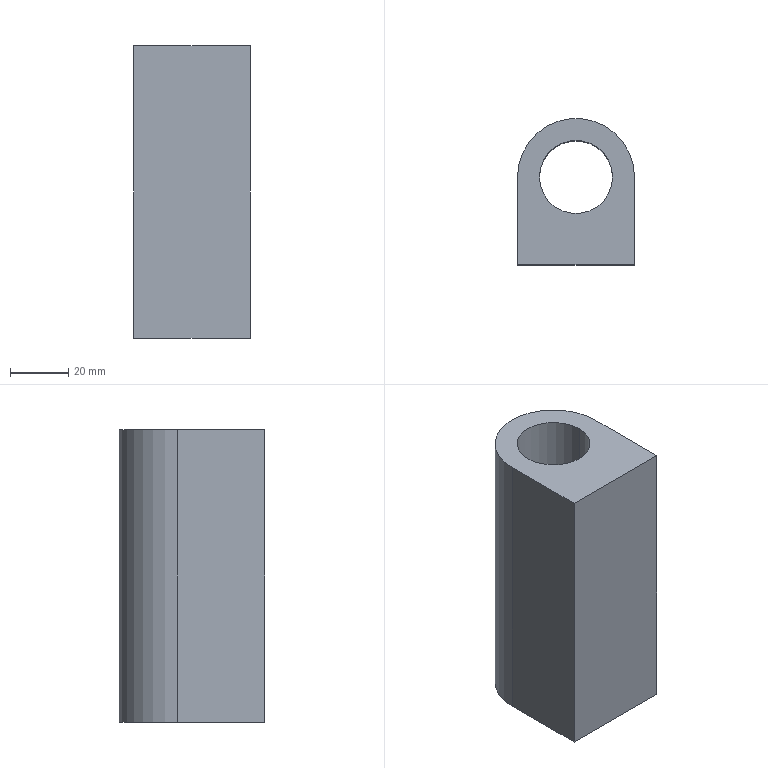Part | STEP file | FZC-000-002 Rotating shaft A | 1 solid | 8 faces | box 40 x 50 x 100 mm | volume 133744 mm3 | plane 5 | cylinder 3 | commonest cylinder face diameters 25 x2 40 x1
STEP:
#1=CARTESIAN_POINT('',(12.5,0.,100.));
#2=VERTEX_POINT('',#1);
#3=CARTESIAN_POINT('',(-12.5,0.,100.));
#4=VERTEX_POINT('',#3);
#5=CARTESIAN_POINT('',(0.,0.,100.));
#6=DIRECTION('',(0.,0.,-1.));
#7=DIRECTION('',(-1.,0.,0.));
#8=AXIS2_PLACEMENT_3D('',#5,#6,#7);
#9=CIRCLE('',#8,12.5);
#10=EDGE_CURVE('',#2,#4,#9,.T.);
#11=ORIENTED_EDGE('',*,*,#10,.F.);
#12=CARTESIAN_POINT('',(12.5,0.,0.));
#13=VERTEX_POINT('',#12);
#14=CARTESIAN_POINT('',(12.5,0.,100.));
#15=DIRECTION('',(0.,0.,-1.));
#16=VECTOR('',#15,1000.);
#17=LINE('',#14,#16);
#18=EDGE_CURVE('',#2,#13,#17,.T.);
#19=ORIENTED_EDGE('',*,*,#18,.T.);
#20=CARTESIAN_POINT('',(-12.5,0.,0.));
#21=VERTEX_POINT('',#20);
#22=CARTESIAN_POINT('',(0.,0.,0.));
#23=DIRECTION('',(0.,0.,-1.));
#24=DIRECTION('',(-1.,0.,0.));
#25=AXIS2_PLACEMENT_3D('',#22,#23,#24);
#26=CIRCLE('',#25,12.5);
#27=EDGE_CURVE('',#13,#21,#26,.T.);
#28=ORIENTED_EDGE('',*,*,#27,.T.);
#29=CARTESIAN_POINT('',(-12.5,0.,100.));
#30=DIRECTION('',(0.,0.,-1.));
#31=VECTOR('',#30,1000.);
#32=LINE('',#29,#31);
#33=EDGE_CURVE('',#4,#21,#32,.T.);
#34=ORIENTED_EDGE('',*,*,#33,.F.);
#35=EDGE_LOOP('',(#11,#19,#28,#34));
#36=FACE_OUTER_BOUND('',#35,.T.);
#37=CARTESIAN_POINT('',(0.,0.,100.));
#38=DIRECTION('',(0.,0.,-1.));
#39=DIRECTION('',(-1.,0.,0.));
#40=AXIS2_PLACEMENT_3D('',#37,#38,#39);
#41=CYLINDRICAL_SURFACE('',#40,12.5);
#42=ADVANCED_FACE('',(#36),#41,.F.);
#43=CARTESIAN_POINT('',(-20.,0.,100.));
#44=VERTEX_POINT('',#43);
#45=CARTESIAN_POINT('',(20.,0.,100.));
#46=VERTEX_POINT('',#45);
#47=CARTESIAN_POINT('',(0.,0.,100.));
#48=DIRECTION('',(0.,0.,-1.));
#49=DIRECTION('',(-1.,0.,0.));
#50=AXIS2_PLACEMENT_3D('',#47,#48,#49);
#51=CIRCLE('',#50,20.);
#52=EDGE_CURVE('',#44,#46,#51,.T.);
#53=ORIENTED_EDGE('',*,*,#52,.T.);
#54=CARTESIAN_POINT('',(20.,0.,0.));
#55=VERTEX_POINT('',#54);
#56=CARTESIAN_POINT('',(20.,0.,100.));
#57=DIRECTION('',(0.,0.,-1.));
#58=VECTOR('',#57,1000.);
#59=LINE('',#56,#58);
#60=EDGE_CURVE('',#46,#55,#59,.T.);
#61=ORIENTED_EDGE('',*,*,#60,.T.);
#62=CARTESIAN_POINT('',(-20.,0.,0.));
#63=VERTEX_POINT('',#62);
#64=CARTESIAN_POINT('',(0.,0.,0.));
#65=DIRECTION('',(0.,0.,1.));
#66=DIRECTION('',(-1.,0.,0.));
#67=AXIS2_PLACEMENT_3D('',#64,#65,#66);
#68=CIRCLE('',#67,20.);
#69=EDGE_CURVE('',#55,#63,#68,.T.);
#70=ORIENTED_EDGE('',*,*,#69,.T.);
#71=CARTESIAN_POINT('',(-20.,0.,100.));
#72=DIRECTION('',(0.,0.,1.));
#73=VECTOR('',#72,1000.);
#74=LINE('',#71,#73);
#75=EDGE_CURVE('',#63,#44,#74,.T.);
#76=ORIENTED_EDGE('',*,*,#75,.T.);
#77=EDGE_LOOP('',(#53,#61,#70,#76));
#78=FACE_OUTER_BOUND('',#77,.T.);
#79=CARTESIAN_POINT('',(0.,0.,100.));
#80=DIRECTION('',(0.,0.,-1.));
#81=DIRECTION('',(-1.,0.,0.));
#82=AXIS2_PLACEMENT_3D('',#79,#80,#81);
#83=CYLINDRICAL_SURFACE('',#82,20.);
#84=ADVANCED_FACE('',(#78),#83,.T.);
#85=ORIENTED_EDGE('',*,*,#60,.F.);
#86=CARTESIAN_POINT('',(20.,-30.,100.));
#87=VERTEX_POINT('',#86);
#88=CARTESIAN_POINT('',(20.,0.,100.));
#89=DIRECTION('',(0.,1.,0.));
#90=VECTOR('',#89,1000.);
#91=LINE('',#88,#90);
#92=EDGE_CURVE('',#87,#46,#91,.T.);
#93=ORIENTED_EDGE('',*,*,#92,.F.);
#94=CARTESIAN_POINT('',(20.,-30.,0.));
#95=VERTEX_POINT('',#94);
#96=CARTESIAN_POINT('',(20.,-30.,100.));
#97=DIRECTION('',(0.,0.,1.));
#98=VECTOR('',#97,1000.);
#99=LINE('',#96,#98);
#100=EDGE_CURVE('',#95,#87,#99,.T.);
#101=ORIENTED_EDGE('',*,*,#100,.F.);
#102=CARTESIAN_POINT('',(20.,0.,0.));
#103=DIRECTION('',(0.,-1.,0.));
#104=VECTOR('',#103,1000.);
#105=LINE('',#102,#104);
#106=EDGE_CURVE('',#55,#95,#105,.T.);
#107=ORIENTED_EDGE('',*,*,#106,.F.);
#108=EDGE_LOOP('',(#85,#93,#101,#107));
#109=FACE_OUTER_BOUND('',#108,.T.);
#110=CARTESIAN_POINT('',(20.,0.,100.));
#111=DIRECTION('',(-1.,0.,0.));
#112=DIRECTION('',(0.,0.,1.));
#113=AXIS2_PLACEMENT_3D('',#110,#111,#112);
#114=PLANE('',#113);
#115=ADVANCED_FACE('',(#109),#114,.F.);
#116=CARTESIAN_POINT('',(0.,0.,100.));
#117=DIRECTION('',(0.,0.,-1.));
#118=DIRECTION('',(-1.,0.,0.));
#119=AXIS2_PLACEMENT_3D('',#116,#117,#118);
#120=CIRCLE('',#119,12.5);
#121=EDGE_CURVE('',#4,#2,#120,.T.);
#122=ORIENTED_EDGE('',*,*,#121,.T.);
#123=ORIENTED_EDGE('',*,*,#10,.T.);
#124=EDGE_LOOP('',(#122,#123));
#125=FACE_BOUND('',#124,.T.);
#126=CARTESIAN_POINT('',(-20.,-30.,100.));
#127=VERTEX_POINT('',#126);
#128=CARTESIAN_POINT('',(0.,-30.,100.));
#129=DIRECTION('',(1.,0.,0.));
#130=VECTOR('',#129,1000.);
#131=LINE('',#128,#130);
#132=EDGE_CURVE('',#127,#87,#131,.T.);
#133=ORIENTED_EDGE('',*,*,#132,.T.);
#134=ORIENTED_EDGE('',*,*,#92,.T.);
#135=ORIENTED_EDGE('',*,*,#52,.F.);
#136=CARTESIAN_POINT('',(-20.,0.,100.));
#137=DIRECTION('',(0.,-1.,0.));
#138=VECTOR('',#137,1000.);
#139=LINE('',#136,#138);
#140=EDGE_CURVE('',#44,#127,#139,.T.);
#141=ORIENTED_EDGE('',*,*,#140,.T.);
#142=EDGE_LOOP('',(#133,#134,#135,#141));
#143=FACE_OUTER_BOUND('',#142,.T.);
#144=CARTESIAN_POINT('',(0.,0.,100.));
#145=DIRECTION('',(0.,0.,1.));
#146=DIRECTION('',(1.,0.,0.));
#147=AXIS2_PLACEMENT_3D('',#144,#145,#146);
#148=PLANE('',#147);
#149=ADVANCED_FACE('',(#125,#143),#148,.T.);
#150=CARTESIAN_POINT('',(-20.,-30.,0.));
#151=VERTEX_POINT('',#150);
#152=CARTESIAN_POINT('',(-20.,-30.,100.));
#153=DIRECTION('',(0.,0.,-1.));
#154=VECTOR('',#153,1000.);
#155=LINE('',#152,#154);
#156=EDGE_CURVE('',#127,#151,#155,.T.);
#157=ORIENTED_EDGE('',*,*,#156,.F.);
#158=ORIENTED_EDGE('',*,*,#140,.F.);
#159=ORIENTED_EDGE('',*,*,#75,.F.);
#160=CARTESIAN_POINT('',(-20.,0.,0.));
#161=DIRECTION('',(0.,1.,0.));
#162=VECTOR('',#161,1000.);
#163=LINE('',#160,#162);
#164=EDGE_CURVE('',#151,#63,#163,.T.);
#165=ORIENTED_EDGE('',*,*,#164,.F.);
#166=EDGE_LOOP('',(#157,#158,#159,#165));
#167=FACE_OUTER_BOUND('',#166,.T.);
#168=CARTESIAN_POINT('',(-20.,0.,100.));
#169=DIRECTION('',(1.,0.,0.));
#170=DIRECTION('',(0.,1.,0.));
#171=AXIS2_PLACEMENT_3D('',#168,#169,#170);
#172=PLANE('',#171);
#173=ADVANCED_FACE('',(#167),#172,.F.);
#174=CARTESIAN_POINT('',(0.,0.,0.));
#175=DIRECTION('',(0.,0.,-1.));
#176=DIRECTION('',(-1.,0.,0.));
#177=AXIS2_PLACEMENT_3D('',#174,#175,#176);
#178=CIRCLE('',#177,12.5);
#179=EDGE_CURVE('',#21,#13,#178,.T.);
#180=ORIENTED_EDGE('',*,*,#179,.F.);
#181=ORIENTED_EDGE('',*,*,#27,.F.);
#182=EDGE_LOOP('',(#180,#181));
#183=FACE_BOUND('',#182,.T.);
#184=ORIENTED_EDGE('',*,*,#106,.T.);
#185=CARTESIAN_POINT('',(0.,-30.,0.));
#186=DIRECTION('',(1.,0.,0.));
#187=VECTOR('',#186,1000.);
#188=LINE('',#185,#187);
#189=EDGE_CURVE('',#151,#95,#188,.T.);
#190=ORIENTED_EDGE('',*,*,#189,.F.);
#191=ORIENTED_EDGE('',*,*,#164,.T.);
#192=ORIENTED_EDGE('',*,*,#69,.F.);
#193=EDGE_LOOP('',(#184,#190,#191,#192));
#194=FACE_OUTER_BOUND('',#193,.T.);
#195=CARTESIAN_POINT('',(0.,0.,0.));
#196=DIRECTION('',(0.,0.,1.));
#197=DIRECTION('',(1.,0.,0.));
#198=AXIS2_PLACEMENT_3D('',#195,#196,#197);
#199=PLANE('',#198);
#200=ADVANCED_FACE('',(#183,#194),#199,.F.);
#201=ORIENTED_EDGE('',*,*,#100,.T.);
#202=ORIENTED_EDGE('',*,*,#132,.F.);
#203=ORIENTED_EDGE('',*,*,#156,.T.);
#204=ORIENTED_EDGE('',*,*,#189,.T.);
#205=EDGE_LOOP('',(#201,#202,#203,#204));
#206=FACE_OUTER_BOUND('',#205,.T.);
#207=CARTESIAN_POINT('',(-20.,-30.,100.));
#208=DIRECTION('',(0.,1.,0.));
#209=DIRECTION('',(0.,0.,1.));
#210=AXIS2_PLACEMENT_3D('',#207,#208,#209);
#211=PLANE('',#210);
#212=ADVANCED_FACE('',(#206),#211,.F.);
#213=ORIENTED_EDGE('',*,*,#18,.F.);
#214=ORIENTED_EDGE('',*,*,#121,.F.);
#215=ORIENTED_EDGE('',*,*,#33,.T.);
#216=ORIENTED_EDGE('',*,*,#179,.T.);
#217=EDGE_LOOP('',(#213,#214,#215,#216));
#218=FACE_OUTER_BOUND('',#217,.T.);
#219=CARTESIAN_POINT('',(0.,0.,100.));
#220=DIRECTION('',(0.,0.,-1.));
#221=DIRECTION('',(-1.,0.,0.));
#222=AXIS2_PLACEMENT_3D('',#219,#220,#221);
#223=CYLINDRICAL_SURFACE('',#222,12.5);
#224=ADVANCED_FACE('',(#218),#223,.F.);
#225=CLOSED_SHELL('',(#42,#84,#115,#149,#173,#200,#212,#224));
#226=MANIFOLD_SOLID_BREP('',#225);
#227=CARTESIAN_POINT('',(0.,0.,0.));
#228=DIRECTION('',(0.,0.,1.));
#229=DIRECTION('',(1.,0.,0.));
#230=AXIS2_PLACEMENT_3D('',#227,#228,#229);
#231=(LENGTH_UNIT()NAMED_UNIT(*)SI_UNIT(.MILLI.,.METRE.));
#232=UNCERTAINTY_MEASURE_WITH_UNIT(LENGTH_MEASURE(0.00001),#231,'','');
#233=(NAMED_UNIT(*)PLANE_ANGLE_UNIT()SI_UNIT($,.RADIAN.));
#234=(NAMED_UNIT(*)SI_UNIT($,.STERADIAN.)SOLID_ANGLE_UNIT());
#235=(GEOMETRIC_REPRESENTATION_CONTEXT(3)GLOBAL_UNCERTAINTY_ASSIGNED_CONTEXT((#232))GLOBAL_UNIT_ASSIGNED_CONTEXT((#231,#233,#234))REPRESENTATION_CONTEXT('',''));
#236=ADVANCED_BREP_SHAPE_REPRESENTATION('',(#226,#230),#235);